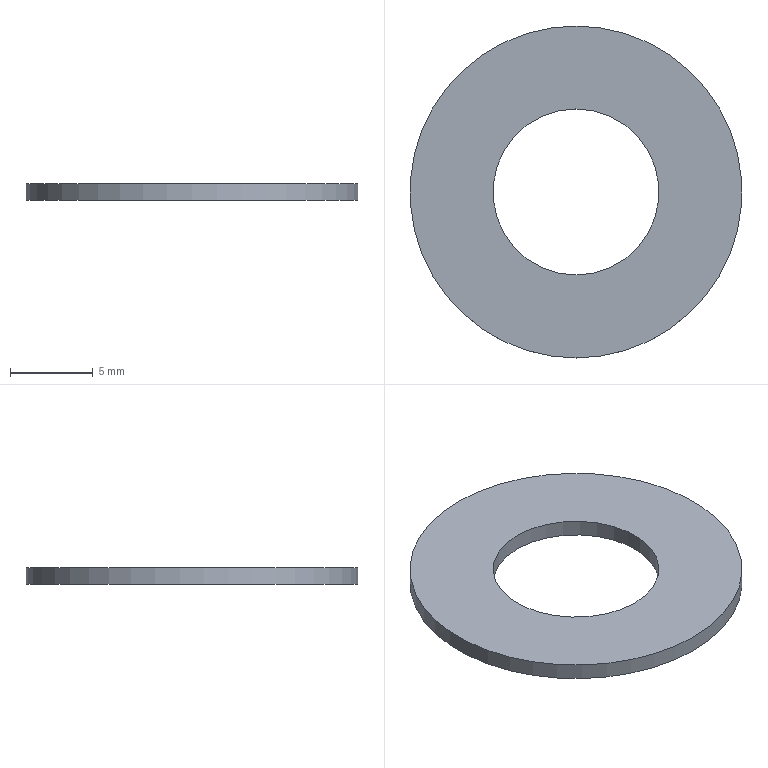Part | STEP file | 1-01.11 | 1 solid | 4 faces | box 20 x 20 x 1 mm | volume 235.619 mm3 | plane 2 | cylinder 2 | commonest cylinder face diameters 10 x1 20 x1
STEP:
#1=CARTESIAN_POINT('',(0.,0.,0.));
#2=DIRECTION('',(0.,0.,1.));
#3=DIRECTION('',(1.,0.,0.));
#4=AXIS2_PLACEMENT_3D('',#1,#2,#3);
#5=CARTESIAN_POINT('',(0.,10.,0.));
#6=VERTEX_POINT('',#5);
#7=CARTESIAN_POINT('',(0.,0.,0.));
#8=DIRECTION('',(0.,0.,1.));
#9=DIRECTION('',(0.,1.,0.));
#10=AXIS2_PLACEMENT_3D('',#7,#8,#9);
#11=CIRCLE('',#10,10.);
#12=CARTESIAN_POINT('',(0.,-2.679,0.));
#13=DIRECTION('',(0.,0.,1.));
#14=DIRECTION('',(0.,1.,0.));
#15=AXIS2_PLACEMENT_3D('',#12,#13,#14);
#16=PLANE('',#15);
#17=CARTESIAN_POINT('',(2.679,0.));
#18=DIRECTION('',(1.,0.));
#19=AXIS2_PLACEMENT_2D('',#17,#18);
#20=CIRCLE('',#19,10.);
#21=(GEOMETRIC_REPRESENTATION_CONTEXT(2)PARAMETRIC_REPRESENTATION_CONTEXT()REPRESENTATION_CONTEXT('',''));
#22=DEFINITIONAL_REPRESENTATION('',(#20),#21);
#23=PCURVE('',#16,#22);
#24=CARTESIAN_POINT('',(0.,0.,0.));
#25=DIRECTION('',(0.,0.,1.));
#26=DIRECTION('',(0.,1.,0.));
#27=AXIS2_PLACEMENT_3D('',#24,#25,#26);
#28=CYLINDRICAL_SURFACE('',#27,10.);
#29=CARTESIAN_POINT('',(0.,0.));
#30=DIRECTION('',(1.,0.));
#31=VECTOR('',#30,1.);
#32=LINE('',#29,#31);
#33=(GEOMETRIC_REPRESENTATION_CONTEXT(2)PARAMETRIC_REPRESENTATION_CONTEXT()REPRESENTATION_CONTEXT('',''));
#34=DEFINITIONAL_REPRESENTATION('',(#32),#33);
#35=PCURVE('',#28,#34);
#36=SURFACE_CURVE('',#11,(#23,#35),.PCURVE_S1.);
#37=EDGE_CURVE('',#6,#6,#36,.T.);
#38=ORIENTED_EDGE('',*,*,#37,.T.);
#39=EDGE_LOOP('',(#38));
#40=FACE_BOUND('',#39,.F.);
#41=CARTESIAN_POINT('',(0.,5.,0.));
#42=VERTEX_POINT('',#41);
#43=CARTESIAN_POINT('',(0.,0.,0.));
#44=DIRECTION('',(0.,0.,-1.));
#45=DIRECTION('',(0.,1.,0.));
#46=AXIS2_PLACEMENT_3D('',#43,#44,#45);
#47=CIRCLE('',#46,5.);
#48=CARTESIAN_POINT('',(7.679,0.));
#49=CARTESIAN_POINT('',(7.679,-8.66));
#50=CARTESIAN_POINT('',(0.1795,-4.33));
#51=CARTESIAN_POINT('',(-7.321,0.));
#52=CARTESIAN_POINT('',(0.1795,4.33));
#53=CARTESIAN_POINT('',(7.679,8.66));
#54=CARTESIAN_POINT('',(7.679,0.));
#55=(BOUNDED_CURVE()B_SPLINE_CURVE(2,(#48,#49,#50,#51,#52,#53,#54),.UNSPECIFIED.,.T.,.F.)B_SPLINE_CURVE_WITH_KNOTS((1,2,2,2,2,1),(-2.094,0.,2.094,4.189,6.283,8.378),.UNSPECIFIED.)CURVE()GEOMETRIC_REPRESENTATION_ITEM()RATIONAL_B_SPLINE_CURVE((1.,0.5,1.,0.5,1.,0.5,1.))REPRESENTATION_ITEM(''));
#56=(GEOMETRIC_REPRESENTATION_CONTEXT(2)PARAMETRIC_REPRESENTATION_CONTEXT()REPRESENTATION_CONTEXT('',''));
#57=DEFINITIONAL_REPRESENTATION('',(#55),#56);
#58=PCURVE('',#16,#57);
#59=CARTESIAN_POINT('',(0.,0.,0.));
#60=DIRECTION('',(0.,0.,1.));
#61=DIRECTION('',(0.,1.,0.));
#62=AXIS2_PLACEMENT_3D('',#59,#60,#61);
#63=CYLINDRICAL_SURFACE('',#62,5.);
#64=CARTESIAN_POINT('',(6.283,0.));
#65=DIRECTION('',(-1.,0.));
#66=VECTOR('',#65,1.);
#67=LINE('',#64,#66);
#68=(GEOMETRIC_REPRESENTATION_CONTEXT(2)PARAMETRIC_REPRESENTATION_CONTEXT()REPRESENTATION_CONTEXT('',''));
#69=DEFINITIONAL_REPRESENTATION('',(#67),#68);
#70=PCURVE('',#63,#69);
#71=SURFACE_CURVE('',#47,(#58,#70),.PCURVE_S1.);
#72=EDGE_CURVE('',#42,#42,#71,.T.);
#73=ORIENTED_EDGE('',*,*,#72,.T.);
#74=EDGE_LOOP('',(#73));
#75=FACE_BOUND('',#74,.F.);
#76=ADVANCED_FACE('',(#40,#75),#16,.F.);
#77=CARTESIAN_POINT('',(0.,10.,1.));
#78=VERTEX_POINT('',#77);
#79=CARTESIAN_POINT('',(0.,0.,1.));
#80=DIRECTION('',(0.,0.,1.));
#81=DIRECTION('',(0.,1.,0.));
#82=AXIS2_PLACEMENT_3D('',#79,#80,#81);
#83=CIRCLE('',#82,10.);
#84=CARTESIAN_POINT('',(0.,-2.679,1.));
#85=DIRECTION('',(0.,0.,1.));
#86=DIRECTION('',(0.,1.,0.));
#87=AXIS2_PLACEMENT_3D('',#84,#85,#86);
#88=PLANE('',#87);
#89=CARTESIAN_POINT('',(2.679,0.));
#90=DIRECTION('',(1.,0.));
#91=AXIS2_PLACEMENT_2D('',#89,#90);
#92=CIRCLE('',#91,10.);
#93=(GEOMETRIC_REPRESENTATION_CONTEXT(2)PARAMETRIC_REPRESENTATION_CONTEXT()REPRESENTATION_CONTEXT('',''));
#94=DEFINITIONAL_REPRESENTATION('',(#92),#93);
#95=PCURVE('',#88,#94);
#96=CARTESIAN_POINT('',(0.,1.));
#97=DIRECTION('',(1.,0.));
#98=VECTOR('',#97,1.);
#99=LINE('',#96,#98);
#100=(GEOMETRIC_REPRESENTATION_CONTEXT(2)PARAMETRIC_REPRESENTATION_CONTEXT()REPRESENTATION_CONTEXT('',''));
#101=DEFINITIONAL_REPRESENTATION('',(#99),#100);
#102=PCURVE('',#28,#101);
#103=SURFACE_CURVE('',#83,(#95,#102),.PCURVE_S1.);
#104=EDGE_CURVE('',#78,#78,#103,.T.);
#105=ORIENTED_EDGE('',*,*,#104,.T.);
#106=EDGE_LOOP('',(#105));
#107=FACE_BOUND('',#106,.T.);
#108=CARTESIAN_POINT('',(0.,5.,1.));
#109=VERTEX_POINT('',#108);
#110=CARTESIAN_POINT('',(0.,0.,1.));
#111=DIRECTION('',(0.,0.,-1.));
#112=DIRECTION('',(0.,1.,0.));
#113=AXIS2_PLACEMENT_3D('',#110,#111,#112);
#114=CIRCLE('',#113,5.);
#115=CARTESIAN_POINT('',(7.679,0.));
#116=CARTESIAN_POINT('',(7.679,-8.66));
#117=CARTESIAN_POINT('',(0.1795,-4.33));
#118=CARTESIAN_POINT('',(-7.321,0.));
#119=CARTESIAN_POINT('',(0.1795,4.33));
#120=CARTESIAN_POINT('',(7.679,8.66));
#121=CARTESIAN_POINT('',(7.679,0.));
#122=(BOUNDED_CURVE()B_SPLINE_CURVE(2,(#115,#116,#117,#118,#119,#120,#121),.UNSPECIFIED.,.T.,.F.)B_SPLINE_CURVE_WITH_KNOTS((1,2,2,2,2,1),(-2.094,0.,2.094,4.189,6.283,8.378),.UNSPECIFIED.)CURVE()GEOMETRIC_REPRESENTATION_ITEM()RATIONAL_B_SPLINE_CURVE((1.,0.5,1.,0.5,1.,0.5,1.))REPRESENTATION_ITEM(''));
#123=(GEOMETRIC_REPRESENTATION_CONTEXT(2)PARAMETRIC_REPRESENTATION_CONTEXT()REPRESENTATION_CONTEXT('',''));
#124=DEFINITIONAL_REPRESENTATION('',(#122),#123);
#125=PCURVE('',#88,#124);
#126=CARTESIAN_POINT('',(6.283,1.));
#127=DIRECTION('',(-1.,0.));
#128=VECTOR('',#127,1.);
#129=LINE('',#126,#128);
#130=(GEOMETRIC_REPRESENTATION_CONTEXT(2)PARAMETRIC_REPRESENTATION_CONTEXT()REPRESENTATION_CONTEXT('',''));
#131=DEFINITIONAL_REPRESENTATION('',(#129),#130);
#132=PCURVE('',#63,#131);
#133=SURFACE_CURVE('',#114,(#125,#132),.PCURVE_S1.);
#134=EDGE_CURVE('',#109,#109,#133,.T.);
#135=ORIENTED_EDGE('',*,*,#134,.T.);
#136=EDGE_LOOP('',(#135));
#137=FACE_BOUND('',#136,.T.);
#138=ADVANCED_FACE('',(#107,#137),#88,.T.);
#139=ORIENTED_EDGE('',*,*,#37,.T.);
#140=CARTESIAN_POINT('',(0.,10.,0.));
#141=DIRECTION('',(0.,0.,1.));
#142=VECTOR('',#141,1.);
#143=LINE('',#140,#142);
#144=CARTESIAN_POINT('',(6.283,0.));
#145=DIRECTION('',(0.,1.));
#146=VECTOR('',#145,1.);
#147=LINE('',#144,#146);
#148=(GEOMETRIC_REPRESENTATION_CONTEXT(2)PARAMETRIC_REPRESENTATION_CONTEXT()REPRESENTATION_CONTEXT('',''));
#149=DEFINITIONAL_REPRESENTATION('',(#147),#148);
#150=PCURVE('',#28,#149);
#151=CARTESIAN_POINT('',(0.,0.));
#152=DIRECTION('',(0.,1.));
#153=VECTOR('',#152,1.);
#154=LINE('',#151,#153);
#155=(GEOMETRIC_REPRESENTATION_CONTEXT(2)PARAMETRIC_REPRESENTATION_CONTEXT()REPRESENTATION_CONTEXT('',''));
#156=DEFINITIONAL_REPRESENTATION('',(#154),#155);
#157=PCURVE('',#28,#156);
#158=SEAM_CURVE('',#143,(#150,#157),.PCURVE_S1.);
#159=EDGE_CURVE('',#6,#78,#158,.T.);
#160=ORIENTED_EDGE('',*,*,#159,.T.);
#161=ORIENTED_EDGE('',*,*,#104,.F.);
#162=ORIENTED_EDGE('',*,*,#159,.F.);
#163=EDGE_LOOP('',(#139,#160,#161,#162));
#164=FACE_BOUND('',#163,.T.);
#165=ADVANCED_FACE('',(#164),#28,.T.);
#166=CARTESIAN_POINT('',(0.,5.,0.));
#167=DIRECTION('',(0.,0.,1.));
#168=VECTOR('',#167,1.);
#169=LINE('',#166,#168);
#170=CARTESIAN_POINT('',(6.283,0.));
#171=DIRECTION('',(0.,1.));
#172=VECTOR('',#171,1.);
#173=LINE('',#170,#172);
#174=(GEOMETRIC_REPRESENTATION_CONTEXT(2)PARAMETRIC_REPRESENTATION_CONTEXT()REPRESENTATION_CONTEXT('',''));
#175=DEFINITIONAL_REPRESENTATION('',(#173),#174);
#176=PCURVE('',#63,#175);
#177=CARTESIAN_POINT('',(0.,0.));
#178=DIRECTION('',(0.,1.));
#179=VECTOR('',#178,1.);
#180=LINE('',#177,#179);
#181=(GEOMETRIC_REPRESENTATION_CONTEXT(2)PARAMETRIC_REPRESENTATION_CONTEXT()REPRESENTATION_CONTEXT('',''));
#182=DEFINITIONAL_REPRESENTATION('',(#180),#181);
#183=PCURVE('',#63,#182);
#184=SEAM_CURVE('',#169,(#176,#183),.PCURVE_S1.);
#185=EDGE_CURVE('',#42,#109,#184,.T.);
#186=ORIENTED_EDGE('',*,*,#185,.T.);
#187=ORIENTED_EDGE('',*,*,#134,.T.);
#188=ORIENTED_EDGE('',*,*,#185,.F.);
#189=ORIENTED_EDGE('',*,*,#72,.F.);
#190=EDGE_LOOP('',(#186,#187,#188,#189));
#191=FACE_BOUND('',#190,.F.);
#192=ADVANCED_FACE('',(#191),#63,.F.);
#193=CLOSED_SHELL('',(#76,#138,#165,#192));
#194=MANIFOLD_SOLID_BREP('',#193);
#195=(LENGTH_UNIT()NAMED_UNIT(*)SI_UNIT(.MILLI.,.METRE.));
#196=UNCERTAINTY_MEASURE_WITH_UNIT(LENGTH_MEASURE(0.0000001),#195,'','');
#197=(NAMED_UNIT(*)PLANE_ANGLE_UNIT()SI_UNIT($,.RADIAN.));
#198=(NAMED_UNIT(*)SI_UNIT($,.STERADIAN.)SOLID_ANGLE_UNIT());
#199=(GEOMETRIC_REPRESENTATION_CONTEXT(3)GLOBAL_UNCERTAINTY_ASSIGNED_CONTEXT((#196))GLOBAL_UNIT_ASSIGNED_CONTEXT((#195,#197,#198))REPRESENTATION_CONTEXT('',''));
#200=ADVANCED_BREP_SHAPE_REPRESENTATION('',(#4,#194),#199);